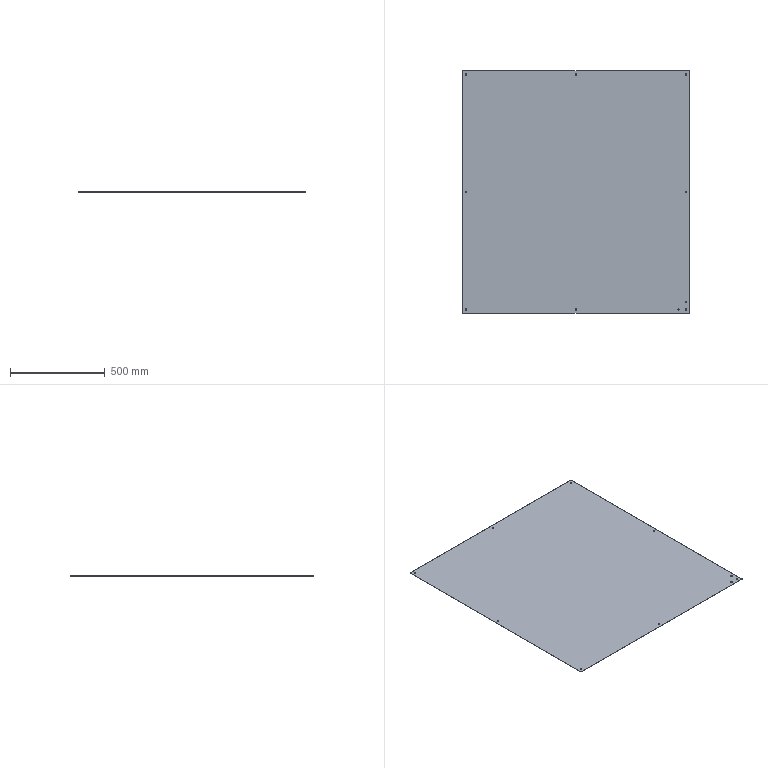Part | SolidWorks | features Fillet 2, HoleWzd 2, FlatPattern 1, SMBaseFlange 1, SheetMetal 1 | 1 solid | 30 faces | box 1200 x 1280 x 1.2 mm | volume 1842780 mm3 | cylinder 24 | plane 6 | commonest cylinder face diameters 6.6 x20 6 x4
STEP:
#1=CARTESIAN_POINT('',(576.7,-580.,-1.2));
#2=VERTEX_POINT('',#1);
#3=CARTESIAN_POINT('',(583.3,-580.,-1.2));
#4=VERTEX_POINT('',#3);
#5=CARTESIAN_POINT('',(580.,-580.,-1.2));
#6=DIRECTION('',(0.,0.,1.));
#7=DIRECTION('',(1.,0.,0.));
#8=AXIS2_PLACEMENT_3D('',#5,#6,#7);
#9=CIRCLE('',#8,3.3);
#10=EDGE_CURVE('',#2,#4,#9,.T.);
#11=ORIENTED_EDGE('',*,*,#10,.F.);
#12=CARTESIAN_POINT('',(576.7,-580.,0.));
#13=VERTEX_POINT('',#12);
#14=CARTESIAN_POINT('',(576.7,-580.,0.));
#15=DIRECTION('',(0.,0.,1.));
#16=VECTOR('',#15,1000.);
#17=LINE('',#14,#16);
#18=EDGE_CURVE('',#2,#13,#17,.T.);
#19=ORIENTED_EDGE('',*,*,#18,.T.);
#20=CARTESIAN_POINT('',(583.3,-580.,0.));
#21=VERTEX_POINT('',#20);
#22=CARTESIAN_POINT('',(580.,-580.,0.));
#23=DIRECTION('',(0.,0.,1.));
#24=DIRECTION('',(1.,0.,0.));
#25=AXIS2_PLACEMENT_3D('',#22,#23,#24);
#26=CIRCLE('',#25,3.3);
#27=EDGE_CURVE('',#13,#21,#26,.T.);
#28=ORIENTED_EDGE('',*,*,#27,.T.);
#29=CARTESIAN_POINT('',(583.3,-580.,0.));
#30=DIRECTION('',(0.,0.,1.));
#31=VECTOR('',#30,1000.);
#32=LINE('',#29,#31);
#33=EDGE_CURVE('',#4,#21,#32,.T.);
#34=ORIENTED_EDGE('',*,*,#33,.F.);
#35=EDGE_LOOP('',(#11,#19,#28,#34));
#36=FACE_OUTER_BOUND('',#35,.T.);
#37=CARTESIAN_POINT('',(580.,-580.,0.));
#38=DIRECTION('',(0.,0.,1.));
#39=DIRECTION('',(1.,0.,0.));
#40=AXIS2_PLACEMENT_3D('',#37,#38,#39);
#41=CYLINDRICAL_SURFACE('',#40,3.3);
#42=ADVANCED_FACE('',(#36),#41,.F.);
#43=CARTESIAN_POINT('',(536.7,-620.,-1.2));
#44=VERTEX_POINT('',#43);
#45=CARTESIAN_POINT('',(543.3,-620.,-1.2));
#46=VERTEX_POINT('',#45);
#47=CARTESIAN_POINT('',(540.,-620.,-1.2));
#48=DIRECTION('',(0.,0.,1.));
#49=DIRECTION('',(1.,0.,0.));
#50=AXIS2_PLACEMENT_3D('',#47,#48,#49);
#51=CIRCLE('',#50,3.3);
#52=EDGE_CURVE('',#44,#46,#51,.T.);
#53=ORIENTED_EDGE('',*,*,#52,.F.);
#54=CARTESIAN_POINT('',(536.7,-620.,0.));
#55=VERTEX_POINT('',#54);
#56=CARTESIAN_POINT('',(536.7,-620.,0.));
#57=DIRECTION('',(0.,0.,1.));
#58=VECTOR('',#57,1000.);
#59=LINE('',#56,#58);
#60=EDGE_CURVE('',#44,#55,#59,.T.);
#61=ORIENTED_EDGE('',*,*,#60,.T.);
#62=CARTESIAN_POINT('',(543.3,-620.,0.));
#63=VERTEX_POINT('',#62);
#64=CARTESIAN_POINT('',(540.,-620.,0.));
#65=DIRECTION('',(0.,0.,1.));
#66=DIRECTION('',(1.,0.,0.));
#67=AXIS2_PLACEMENT_3D('',#64,#65,#66);
#68=CIRCLE('',#67,3.3);
#69=EDGE_CURVE('',#55,#63,#68,.T.);
#70=ORIENTED_EDGE('',*,*,#69,.T.);
#71=CARTESIAN_POINT('',(543.3,-620.,0.));
#72=DIRECTION('',(0.,0.,1.));
#73=VECTOR('',#72,1000.);
#74=LINE('',#71,#73);
#75=EDGE_CURVE('',#46,#63,#74,.T.);
#76=ORIENTED_EDGE('',*,*,#75,.F.);
#77=EDGE_LOOP('',(#53,#61,#70,#76));
#78=FACE_OUTER_BOUND('',#77,.T.);
#79=CARTESIAN_POINT('',(540.,-620.,0.));
#80=DIRECTION('',(0.,0.,1.));
#81=DIRECTION('',(1.,0.,0.));
#82=AXIS2_PLACEMENT_3D('',#79,#80,#81);
#83=CYLINDRICAL_SURFACE('',#82,3.3);
#84=ADVANCED_FACE('',(#78),#83,.F.);
#85=CARTESIAN_POINT('',(-583.3,620.,-1.2));
#86=VERTEX_POINT('',#85);
#87=CARTESIAN_POINT('',(-576.7,620.,-1.2));
#88=VERTEX_POINT('',#87);
#89=CARTESIAN_POINT('',(-580.,620.,-1.2));
#90=DIRECTION('',(0.,0.,1.));
#91=DIRECTION('',(1.,0.,0.));
#92=AXIS2_PLACEMENT_3D('',#89,#90,#91);
#93=CIRCLE('',#92,3.3);
#94=EDGE_CURVE('',#86,#88,#93,.T.);
#95=ORIENTED_EDGE('',*,*,#94,.F.);
#96=CARTESIAN_POINT('',(-583.3,620.,0.));
#97=VERTEX_POINT('',#96);
#98=CARTESIAN_POINT('',(-583.3,620.,0.));
#99=DIRECTION('',(0.,0.,1.));
#100=VECTOR('',#99,1000.);
#101=LINE('',#98,#100);
#102=EDGE_CURVE('',#86,#97,#101,.T.);
#103=ORIENTED_EDGE('',*,*,#102,.T.);
#104=CARTESIAN_POINT('',(-576.7,620.,0.));
#105=VERTEX_POINT('',#104);
#106=CARTESIAN_POINT('',(-580.,620.,0.));
#107=DIRECTION('',(0.,0.,1.));
#108=DIRECTION('',(1.,0.,0.));
#109=AXIS2_PLACEMENT_3D('',#106,#107,#108);
#110=CIRCLE('',#109,3.3);
#111=EDGE_CURVE('',#97,#105,#110,.T.);
#112=ORIENTED_EDGE('',*,*,#111,.T.);
#113=CARTESIAN_POINT('',(-576.7,620.,0.));
#114=DIRECTION('',(0.,0.,1.));
#115=VECTOR('',#114,1000.);
#116=LINE('',#113,#115);
#117=EDGE_CURVE('',#88,#105,#116,.T.);
#118=ORIENTED_EDGE('',*,*,#117,.F.);
#119=EDGE_LOOP('',(#95,#103,#112,#118));
#120=FACE_OUTER_BOUND('',#119,.T.);
#121=CARTESIAN_POINT('',(-580.,620.,0.));
#122=DIRECTION('',(0.,0.,1.));
#123=DIRECTION('',(1.,0.,0.));
#124=AXIS2_PLACEMENT_3D('',#121,#122,#123);
#125=CYLINDRICAL_SURFACE('',#124,3.3);
#126=ADVANCED_FACE('',(#120),#125,.F.);
#127=CARTESIAN_POINT('',(-3.3,620.,-1.2));
#128=VERTEX_POINT('',#127);
#129=CARTESIAN_POINT('',(3.3,620.,-1.2));
#130=VERTEX_POINT('',#129);
#131=CARTESIAN_POINT('',(0.,620.,-1.2));
#132=DIRECTION('',(0.,0.,1.));
#133=DIRECTION('',(1.,0.,0.));
#134=AXIS2_PLACEMENT_3D('',#131,#132,#133);
#135=CIRCLE('',#134,3.3);
#136=EDGE_CURVE('',#128,#130,#135,.T.);
#137=ORIENTED_EDGE('',*,*,#136,.F.);
#138=CARTESIAN_POINT('',(-3.3,620.,0.));
#139=VERTEX_POINT('',#138);
#140=CARTESIAN_POINT('',(-3.3,620.,0.));
#141=DIRECTION('',(0.,0.,1.));
#142=VECTOR('',#141,1000.);
#143=LINE('',#140,#142);
#144=EDGE_CURVE('',#128,#139,#143,.T.);
#145=ORIENTED_EDGE('',*,*,#144,.T.);
#146=CARTESIAN_POINT('',(3.3,620.,0.));
#147=VERTEX_POINT('',#146);
#148=CARTESIAN_POINT('',(0.,620.,0.));
#149=DIRECTION('',(0.,0.,1.));
#150=DIRECTION('',(1.,0.,0.));
#151=AXIS2_PLACEMENT_3D('',#148,#149,#150);
#152=CIRCLE('',#151,3.3);
#153=EDGE_CURVE('',#139,#147,#152,.T.);
#154=ORIENTED_EDGE('',*,*,#153,.T.);
#155=CARTESIAN_POINT('',(3.3,620.,0.));
#156=DIRECTION('',(0.,0.,1.));
#157=VECTOR('',#156,1000.);
#158=LINE('',#155,#157);
#159=EDGE_CURVE('',#130,#147,#158,.T.);
#160=ORIENTED_EDGE('',*,*,#159,.F.);
#161=EDGE_LOOP('',(#137,#145,#154,#160));
#162=FACE_OUTER_BOUND('',#161,.T.);
#163=CARTESIAN_POINT('',(0.,620.,0.));
#164=DIRECTION('',(0.,0.,1.));
#165=DIRECTION('',(1.,0.,0.));
#166=AXIS2_PLACEMENT_3D('',#163,#164,#165);
#167=CYLINDRICAL_SURFACE('',#166,3.3);
#168=ADVANCED_FACE('',(#162),#167,.F.);
#169=CARTESIAN_POINT('',(576.7,620.,-1.2));
#170=VERTEX_POINT('',#169);
#171=CARTESIAN_POINT('',(583.3,620.,-1.2));
#172=VERTEX_POINT('',#171);
#173=CARTESIAN_POINT('',(580.,620.,-1.2));
#174=DIRECTION('',(0.,0.,1.));
#175=DIRECTION('',(1.,0.,0.));
#176=AXIS2_PLACEMENT_3D('',#173,#174,#175);
#177=CIRCLE('',#176,3.3);
#178=EDGE_CURVE('',#170,#172,#177,.T.);
#179=ORIENTED_EDGE('',*,*,#178,.F.);
#180=CARTESIAN_POINT('',(576.7,620.,0.));
#181=VERTEX_POINT('',#180);
#182=CARTESIAN_POINT('',(576.7,620.,0.));
#183=DIRECTION('',(0.,0.,1.));
#184=VECTOR('',#183,1000.);
#185=LINE('',#182,#184);
#186=EDGE_CURVE('',#170,#181,#185,.T.);
#187=ORIENTED_EDGE('',*,*,#186,.T.);
#188=CARTESIAN_POINT('',(583.3,620.,0.));
#189=VERTEX_POINT('',#188);
#190=CARTESIAN_POINT('',(580.,620.,0.));
#191=DIRECTION('',(0.,0.,1.));
#192=DIRECTION('',(1.,0.,0.));
#193=AXIS2_PLACEMENT_3D('',#190,#191,#192);
#194=CIRCLE('',#193,3.3);
#195=EDGE_CURVE('',#181,#189,#194,.T.);
#196=ORIENTED_EDGE('',*,*,#195,.T.);
#197=CARTESIAN_POINT('',(583.3,620.,0.));
#198=DIRECTION('',(0.,0.,1.));
#199=VECTOR('',#198,1000.);
#200=LINE('',#197,#199);
#201=EDGE_CURVE('',#172,#189,#200,.T.);
#202=ORIENTED_EDGE('',*,*,#201,.F.);
#203=EDGE_LOOP('',(#179,#187,#196,#202));
#204=FACE_OUTER_BOUND('',#203,.T.);
#205=CARTESIAN_POINT('',(580.,620.,0.));
#206=DIRECTION('',(0.,0.,1.));
#207=DIRECTION('',(1.,0.,0.));
#208=AXIS2_PLACEMENT_3D('',#205,#206,#207);
#209=CYLINDRICAL_SURFACE('',#208,3.3);
#210=ADVANCED_FACE('',(#204),#209,.F.);
#211=CARTESIAN_POINT('',(576.7,0.,-1.2));
#212=VERTEX_POINT('',#211);
#213=CARTESIAN_POINT('',(583.3,0.,-1.2));
#214=VERTEX_POINT('',#213);
#215=CARTESIAN_POINT('',(580.,0.,-1.2));
#216=DIRECTION('',(0.,0.,1.));
#217=DIRECTION('',(1.,0.,0.));
#218=AXIS2_PLACEMENT_3D('',#215,#216,#217);
#219=CIRCLE('',#218,3.3);
#220=EDGE_CURVE('',#212,#214,#219,.T.);
#221=ORIENTED_EDGE('',*,*,#220,.F.);
#222=CARTESIAN_POINT('',(576.7,0.,0.));
#223=VERTEX_POINT('',#222);
#224=CARTESIAN_POINT('',(576.7,0.,0.));
#225=DIRECTION('',(0.,0.,1.));
#226=VECTOR('',#225,1000.);
#227=LINE('',#224,#226);
#228=EDGE_CURVE('',#212,#223,#227,.T.);
#229=ORIENTED_EDGE('',*,*,#228,.T.);
#230=CARTESIAN_POINT('',(583.3,0.,0.));
#231=VERTEX_POINT('',#230);
#232=CARTESIAN_POINT('',(580.,0.,0.));
#233=DIRECTION('',(0.,0.,1.));
#234=DIRECTION('',(1.,0.,0.));
#235=AXIS2_PLACEMENT_3D('',#232,#233,#234);
#236=CIRCLE('',#235,3.3);
#237=EDGE_CURVE('',#223,#231,#236,.T.);
#238=ORIENTED_EDGE('',*,*,#237,.T.);
#239=CARTESIAN_POINT('',(583.3,0.,0.));
#240=DIRECTION('',(0.,0.,1.));
#241=VECTOR('',#240,1000.);
#242=LINE('',#239,#241);
#243=EDGE_CURVE('',#214,#231,#242,.T.);
#244=ORIENTED_EDGE('',*,*,#243,.F.);
#245=EDGE_LOOP('',(#221,#229,#238,#244));
#246=FACE_OUTER_BOUND('',#245,.T.);
#247=CARTESIAN_POINT('',(580.,0.,0.));
#248=DIRECTION('',(0.,0.,1.));
#249=DIRECTION('',(1.,0.,0.));
#250=AXIS2_PLACEMENT_3D('',#247,#248,#249);
#251=CYLINDRICAL_SURFACE('',#250,3.3);
#252=ADVANCED_FACE('',(#246),#251,.F.);
#253=CARTESIAN_POINT('',(576.7,-620.,-1.2));
#254=VERTEX_POINT('',#253);
#255=CARTESIAN_POINT('',(583.3,-620.,-1.2));
#256=VERTEX_POINT('',#255);
#257=CARTESIAN_POINT('',(580.,-620.,-1.2));
#258=DIRECTION('',(0.,0.,1.));
#259=DIRECTION('',(1.,0.,0.));
#260=AXIS2_PLACEMENT_3D('',#257,#258,#259);
#261=CIRCLE('',#260,3.3);
#262=EDGE_CURVE('',#254,#256,#261,.T.);
#263=ORIENTED_EDGE('',*,*,#262,.F.);
#264=CARTESIAN_POINT('',(576.7,-620.,0.));
#265=VERTEX_POINT('',#264);
#266=CARTESIAN_POINT('',(576.7,-620.,0.));
#267=DIRECTION('',(0.,0.,1.));
#268=VECTOR('',#267,1000.);
#269=LINE('',#266,#268);
#270=EDGE_CURVE('',#254,#265,#269,.T.);
#271=ORIENTED_EDGE('',*,*,#270,.T.);
#272=CARTESIAN_POINT('',(583.3,-620.,0.));
#273=VERTEX_POINT('',#272);
#274=CARTESIAN_POINT('',(580.,-620.,0.));
#275=DIRECTION('',(0.,0.,1.));
#276=DIRECTION('',(1.,0.,0.));
#277=AXIS2_PLACEMENT_3D('',#274,#275,#276);
#278=CIRCLE('',#277,3.3);
#279=EDGE_CURVE('',#265,#273,#278,.T.);
#280=ORIENTED_EDGE('',*,*,#279,.T.);
#281=CARTESIAN_POINT('',(583.3,-620.,0.));
#282=DIRECTION('',(0.,0.,1.));
#283=VECTOR('',#282,1000.);
#284=LINE('',#281,#283);
#285=EDGE_CURVE('',#256,#273,#284,.T.);
#286=ORIENTED_EDGE('',*,*,#285,.F.);
#287=EDGE_LOOP('',(#263,#271,#280,#286));
#288=FACE_OUTER_BOUND('',#287,.T.);
#289=CARTESIAN_POINT('',(580.,-620.,0.));
#290=DIRECTION('',(0.,0.,1.));
#291=DIRECTION('',(1.,0.,0.));
#292=AXIS2_PLACEMENT_3D('',#289,#290,#291);
#293=CYLINDRICAL_SURFACE('',#292,3.3);
#294=ADVANCED_FACE('',(#288),#293,.F.);
#295=CARTESIAN_POINT('',(-3.3,-620.,-1.2));
#296=VERTEX_POINT('',#295);
#297=CARTESIAN_POINT('',(3.3,-620.,-1.2));
#298=VERTEX_POINT('',#297);
#299=CARTESIAN_POINT('',(0.,-620.,-1.2));
#300=DIRECTION('',(0.,0.,1.));
#301=DIRECTION('',(1.,0.,0.));
#302=AXIS2_PLACEMENT_3D('',#299,#300,#301);
#303=CIRCLE('',#302,3.3);
#304=EDGE_CURVE('',#296,#298,#303,.T.);
#305=ORIENTED_EDGE('',*,*,#304,.F.);
#306=CARTESIAN_POINT('',(-3.3,-620.,0.));
#307=VERTEX_POINT('',#306);
#308=CARTESIAN_POINT('',(-3.3,-620.,0.));
#309=DIRECTION('',(0.,0.,1.));
#310=VECTOR('',#309,1000.);
#311=LINE('',#308,#310);
#312=EDGE_CURVE('',#296,#307,#311,.T.);
#313=ORIENTED_EDGE('',*,*,#312,.T.);
#314=CARTESIAN_POINT('',(3.3,-620.,0.));
#315=VERTEX_POINT('',#314);
#316=CARTESIAN_POINT('',(0.,-620.,0.));
#317=DIRECTION('',(0.,0.,1.));
#318=DIRECTION('',(1.,0.,0.));
#319=AXIS2_PLACEMENT_3D('',#316,#317,#318);
#320=CIRCLE('',#319,3.3);
#321=EDGE_CURVE('',#307,#315,#320,.T.);
#322=ORIENTED_EDGE('',*,*,#321,.T.);
#323=CARTESIAN_POINT('',(3.3,-620.,0.));
#324=DIRECTION('',(0.,0.,1.));
#325=VECTOR('',#324,1000.);
#326=LINE('',#323,#325);
#327=EDGE_CURVE('',#298,#315,#326,.T.);
#328=ORIENTED_EDGE('',*,*,#327,.F.);
#329=EDGE_LOOP('',(#305,#313,#322,#328));
#330=FACE_OUTER_BOUND('',#329,.T.);
#331=CARTESIAN_POINT('',(0.,-620.,0.));
#332=DIRECTION('',(0.,0.,1.));
#333=DIRECTION('',(1.,0.,0.));
#334=AXIS2_PLACEMENT_3D('',#331,#332,#333);
#335=CYLINDRICAL_SURFACE('',#334,3.3);
#336=ADVANCED_FACE('',(#330),#335,.F.);
#337=CARTESIAN_POINT('',(-583.3,-620.,-1.2));
#338=VERTEX_POINT('',#337);
#339=CARTESIAN_POINT('',(-576.7,-620.,-1.2));
#340=VERTEX_POINT('',#339);
#341=CARTESIAN_POINT('',(-580.,-620.,-1.2));
#342=DIRECTION('',(0.,0.,1.));
#343=DIRECTION('',(1.,0.,0.));
#344=AXIS2_PLACEMENT_3D('',#341,#342,#343);
#345=CIRCLE('',#344,3.3);
#346=EDGE_CURVE('',#338,#340,#345,.T.);
#347=ORIENTED_EDGE('',*,*,#346,.F.);
#348=CARTESIAN_POINT('',(-583.3,-620.,0.));
#349=VERTEX_POINT('',#348);
#350=CARTESIAN_POINT('',(-583.3,-620.,0.));
#351=DIRECTION('',(0.,0.,1.));
#352=VECTOR('',#351,1000.);
#353=LINE('',#350,#352);
#354=EDGE_CURVE('',#338,#349,#353,.T.);
#355=ORIENTED_EDGE('',*,*,#354,.T.);
#356=CARTESIAN_POINT('',(-576.7,-620.,0.));
#357=VERTEX_POINT('',#356);
#358=CARTESIAN_POINT('',(-580.,-620.,0.));
#359=DIRECTION('',(0.,0.,1.));
#360=DIRECTION('',(1.,0.,0.));
#361=AXIS2_PLACEMENT_3D('',#358,#359,#360);
#362=CIRCLE('',#361,3.3);
#363=EDGE_CURVE('',#349,#357,#362,.T.);
#364=ORIENTED_EDGE('',*,*,#363,.T.);
#365=CARTESIAN_POINT('',(-576.7,-620.,0.));
#366=DIRECTION('',(0.,0.,1.));
#367=VECTOR('',#366,1000.);
#368=LINE('',#365,#367);
#369=EDGE_CURVE('',#340,#357,#368,.T.);
#370=ORIENTED_EDGE('',*,*,#369,.F.);
#371=EDGE_LOOP('',(#347,#355,#364,#370));
#372=FACE_OUTER_BOUND('',#371,.T.);
#373=CARTESIAN_POINT('',(-580.,-620.,0.));
#374=DIRECTION('',(0.,0.,1.));
#375=DIRECTION('',(1.,0.,0.));
#376=AXIS2_PLACEMENT_3D('',#373,#374,#375);
#377=CYLINDRICAL_SURFACE('',#376,3.3);
#378=ADVANCED_FACE('',(#372),#377,.F.);
#379=CARTESIAN_POINT('',(-583.3,0.,-1.2));
#380=VERTEX_POINT('',#379);
#381=CARTESIAN_POINT('',(-576.7,0.,-1.2));
#382=VERTEX_POINT('',#381);
#383=CARTESIAN_POINT('',(-580.,0.,-1.2));
#384=DIRECTION('',(0.,0.,1.));
#385=DIRECTION('',(1.,0.,0.));
#386=AXIS2_PLACEMENT_3D('',#383,#384,#385);
#387=CIRCLE('',#386,3.3);
#388=EDGE_CURVE('',#380,#382,#387,.T.);
#389=ORIENTED_EDGE('',*,*,#388,.F.);
#390=CARTESIAN_POINT('',(-583.3,0.,0.));
#391=VERTEX_POINT('',#390);
#392=CARTESIAN_POINT('',(-583.3,0.,0.));
#393=DIRECTION('',(0.,0.,1.));
#394=VECTOR('',#393,1000.);
#395=LINE('',#392,#394);
#396=EDGE_CURVE('',#380,#391,#395,.T.);
#397=ORIENTED_EDGE('',*,*,#396,.T.);
#398=CARTESIAN_POINT('',(-576.7,0.,0.));
#399=VERTEX_POINT('',#398);
#400=CARTESIAN_POINT('',(-580.,0.,0.));
#401=DIRECTION('',(0.,0.,1.));
#402=DIRECTION('',(1.,0.,0.));
#403=AXIS2_PLACEMENT_3D('',#400,#401,#402);
#404=CIRCLE('',#403,3.3);
#405=EDGE_CURVE('',#391,#399,#404,.T.);
#406=ORIENTED_EDGE('',*,*,#405,.T.);
#407=CARTESIAN_POINT('',(-576.7,0.,0.));
#408=DIRECTION('',(0.,0.,1.));
#409=VECTOR('',#408,1000.);
#410=LINE('',#407,#409);
#411=EDGE_CURVE('',#382,#399,#410,.T.);
#412=ORIENTED_EDGE('',*,*,#411,.F.);
#413=EDGE_LOOP('',(#389,#397,#406,#412));
#414=FACE_OUTER_BOUND('',#413,.T.);
#415=CARTESIAN_POINT('',(-580.,0.,0.));
#416=DIRECTION('',(0.,0.,1.));
#417=DIRECTION('',(1.,0.,0.));
#418=AXIS2_PLACEMENT_3D('',#415,#416,#417);
#419=CYLINDRICAL_SURFACE('',#418,3.3);
#420=ADVANCED_FACE('',(#414),#419,.F.);
#421=CARTESIAN_POINT('',(600.,-637.,-1.2));
#422=VERTEX_POINT('',#421);
#423=CARTESIAN_POINT('',(600.,637.,-1.2));
#424=VERTEX_POINT('',#423);
#425=CARTESIAN_POINT('',(600.,640.,-1.2));
#426=DIRECTION('',(0.,1.,0.));
#427=VECTOR('',#426,1000.);
#428=LINE('',#425,#427);
#429=EDGE_CURVE('',#422,#424,#428,.T.);
#430=ORIENTED_EDGE('',*,*,#429,.T.);
#431=CARTESIAN_POINT('',(600.,637.,0.));
#432=VERTEX_POINT('',#431);
#433=CARTESIAN_POINT('',(600.,637.,-1.2));
#434=DIRECTION('',(0.,0.,1.));
#435=VECTOR('',#434,1000.);
#436=LINE('',#433,#435);
#437=EDGE_CURVE('',#424,#432,#436,.T.);
#438=ORIENTED_EDGE('',*,*,#437,.T.);
#439=CARTESIAN_POINT('',(600.,-637.,0.));
#440=VERTEX_POINT('',#439);
#441=CARTESIAN_POINT('',(600.,640.,0.));
#442=DIRECTION('',(0.,1.,0.));
#443=VECTOR('',#442,1000.);
#444=LINE('',#441,#443);
#445=EDGE_CURVE('',#440,#432,#444,.T.);
#446=ORIENTED_EDGE('',*,*,#445,.F.);
#447=CARTESIAN_POINT('',(600.,-637.,-1.2));
#448=DIRECTION('',(0.,0.,-1.));
#449=VECTOR('',#448,1000.);
#450=LINE('',#447,#449);
#451=EDGE_CURVE('',#440,#422,#450,.T.);
#452=ORIENTED_EDGE('',*,*,#451,.T.);
#453=EDGE_LOOP('',(#430,#438,#446,#452));
#454=FACE_OUTER_BOUND('',#453,.T.);
#455=CARTESIAN_POINT('',(600.,640.,-1.2));
#456=DIRECTION('',(1.,0.,0.));
#457=DIRECTION('',(0.,0.,-1.));
#458=AXIS2_PLACEMENT_3D('',#455,#456,#457);
#459=PLANE('',#458);
#460=ADVANCED_FACE('',(#454),#459,.T.);
#461=CARTESIAN_POINT('',(-597.,-640.,-1.2));
#462=VERTEX_POINT('',#461);
#463=CARTESIAN_POINT('',(597.,-640.,-1.2));
#464=VERTEX_POINT('',#463);
#465=CARTESIAN_POINT('',(-600.,-640.,-1.2));
#466=DIRECTION('',(1.,0.,0.));
#467=VECTOR('',#466,1000.);
#468=LINE('',#465,#467);
#469=EDGE_CURVE('',#462,#464,#468,.T.);
#470=ORIENTED_EDGE('',*,*,#469,.T.);
#471=CARTESIAN_POINT('',(597.,-640.,0.));
#472=VERTEX_POINT('',#471);
#473=CARTESIAN_POINT('',(597.,-640.,-1.2));
#474=DIRECTION('',(0.,0.,1.));
#475=VECTOR('',#474,1000.);
#476=LINE('',#473,#475);
#477=EDGE_CURVE('',#464,#472,#476,.T.);
#478=ORIENTED_EDGE('',*,*,#477,.T.);
#479=CARTESIAN_POINT('',(-597.,-640.,0.));
#480=VERTEX_POINT('',#479);
#481=CARTESIAN_POINT('',(-600.,-640.,0.));
#482=DIRECTION('',(1.,0.,0.));
#483=VECTOR('',#482,1000.);
#484=LINE('',#481,#483);
#485=EDGE_CURVE('',#480,#472,#484,.T.);
#486=ORIENTED_EDGE('',*,*,#485,.F.);
#487=CARTESIAN_POINT('',(-597.,-640.,-1.2));
#488=DIRECTION('',(0.,0.,-1.));
#489=VECTOR('',#488,1000.);
#490=LINE('',#487,#489);
#491=EDGE_CURVE('',#480,#462,#490,.T.);
#492=ORIENTED_EDGE('',*,*,#491,.T.);
#493=EDGE_LOOP('',(#470,#478,#486,#492));
#494=FACE_OUTER_BOUND('',#493,.T.);
#495=CARTESIAN_POINT('',(-600.,-640.,-1.2));
#496=DIRECTION('',(0.,-1.,0.));
#497=DIRECTION('',(0.,0.,-1.));
#498=AXIS2_PLACEMENT_3D('',#495,#496,#497);
#499=PLANE('',#498);
#500=ADVANCED_FACE('',(#494),#499,.T.);
#501=CARTESIAN_POINT('',(-600.,637.,0.));
#502=VERTEX_POINT('',#501);
#503=CARTESIAN_POINT('',(-600.,-637.,0.));
#504=VERTEX_POINT('',#503);
#505=CARTESIAN_POINT('',(-600.,640.,0.));
#506=DIRECTION('',(0.,-1.,0.));
#507=VECTOR('',#506,1000.);
#508=LINE('',#505,#507);
#509=EDGE_CURVE('',#502,#504,#508,.T.);
#510=ORIENTED_EDGE('',*,*,#509,.F.);
#511=CARTESIAN_POINT('',(-600.,637.,-1.2));
#512=VERTEX_POINT('',#511);
#513=CARTESIAN_POINT('',(-600.,637.,-1.2));
#514=DIRECTION('',(0.,0.,-1.));
#515=VECTOR('',#514,1000.);
#516=LINE('',#513,#515);
#517=EDGE_CURVE('',#502,#512,#516,.T.);
#518=ORIENTED_EDGE('',*,*,#517,.T.);
#519=CARTESIAN_POINT('',(-600.,-637.,-1.2));
#520=VERTEX_POINT('',#519);
#521=CARTESIAN_POINT('',(-600.,640.,-1.2));
#522=DIRECTION('',(0.,-1.,0.));
#523=VECTOR('',#522,1000.);
#524=LINE('',#521,#523);
#525=EDGE_CURVE('',#512,#520,#524,.T.);
#526=ORIENTED_EDGE('',*,*,#525,.T.);
#527=CARTESIAN_POINT('',(-600.,-637.,-1.2));
#528=DIRECTION('',(0.,0.,1.));
#529=VECTOR('',#528,1000.);
#530=LINE('',#527,#529);
#531=EDGE_CURVE('',#520,#504,#530,.T.);
#532=ORIENTED_EDGE('',*,*,#531,.T.);
#533=EDGE_LOOP('',(#510,#518,#526,#532));
#534=FACE_OUTER_BOUND('',#533,.T.);
#535=CARTESIAN_POINT('',(-600.,640.,-1.2));
#536=DIRECTION('',(-1.,0.,0.));
#537=DIRECTION('',(0.,-1.,0.));
#538=AXIS2_PLACEMENT_3D('',#535,#536,#537);
#539=PLANE('',#538);
#540=ADVANCED_FACE('',(#534),#539,.T.);
#541=CARTESIAN_POINT('',(597.,640.,-1.2));
#542=VERTEX_POINT('',#541);
#543=CARTESIAN_POINT('',(-597.,640.,-1.2));
#544=VERTEX_POINT('',#543);
#545=CARTESIAN_POINT('',(-600.,640.,-1.2));
#546=DIRECTION('',(-1.,0.,0.));
#547=VECTOR('',#546,1000.);
#548=LINE('',#545,#547);
#549=EDGE_CURVE('',#542,#544,#548,.T.);
#550=ORIENTED_EDGE('',*,*,#549,.T.);
#551=CARTESIAN_POINT('',(-597.,640.,0.));
#552=VERTEX_POINT('',#551);
#553=CARTESIAN_POINT('',(-597.,640.,-1.2));
#554=DIRECTION('',(0.,0.,1.));
#555=VECTOR('',#554,1000.);
#556=LINE('',#553,#555);
#557=EDGE_CURVE('',#544,#552,#556,.T.);
#558=ORIENTED_EDGE('',*,*,#557,.T.);
#559=CARTESIAN_POINT('',(597.,640.,0.));
#560=VERTEX_POINT('',#559);
#561=CARTESIAN_POINT('',(-600.,640.,0.));
#562=DIRECTION('',(-1.,0.,0.));
#563=VECTOR('',#562,1000.);
#564=LINE('',#561,#563);
#565=EDGE_CURVE('',#560,#552,#564,.T.);
#566=ORIENTED_EDGE('',*,*,#565,.F.);
#567=CARTESIAN_POINT('',(597.,640.,-1.2));
#568=DIRECTION('',(0.,0.,-1.));
#569=VECTOR('',#568,1000.);
#570=LINE('',#567,#569);
#571=EDGE_CURVE('',#560,#542,#570,.T.);
#572=ORIENTED_EDGE('',*,*,#571,.T.);
#573=EDGE_LOOP('',(#550,#558,#566,#572));
#574=FACE_OUTER_BOUND('',#573,.T.);
#575=CARTESIAN_POINT('',(-600.,640.,-1.2));
#576=DIRECTION('',(0.,1.,0.));
#577=DIRECTION('',(0.,0.,1.));
#578=AXIS2_PLACEMENT_3D('',#575,#576,#577);
#579=PLANE('',#578);
#580=ADVANCED_FACE('',(#574),#579,.T.);
#581=CARTESIAN_POINT('',(580.,-580.,-1.2));
#582=DIRECTION('',(0.,0.,1.));
#583=DIRECTION('',(1.,0.,0.));
#584=AXIS2_PLACEMENT_3D('',#581,#582,#583);
#585=CIRCLE('',#584,3.3);
#586=EDGE_CURVE('',#4,#2,#585,.T.);
#587=ORIENTED_EDGE('',*,*,#586,.T.);
#588=ORIENTED_EDGE('',*,*,#10,.T.);
#589=EDGE_LOOP('',(#587,#588));
#590=FACE_BOUND('',#589,.T.);
#591=CARTESIAN_POINT('',(540.,-620.,-1.2));
#592=DIRECTION('',(0.,0.,1.));
#593=DIRECTION('',(1.,0.,0.));
#594=AXIS2_PLACEMENT_3D('',#591,#592,#593);
#595=CIRCLE('',#594,3.3);
#596=EDGE_CURVE('',#46,#44,#595,.T.);
#597=ORIENTED_EDGE('',*,*,#596,.T.);
#598=ORIENTED_EDGE('',*,*,#52,.T.);
#599=EDGE_LOOP('',(#597,#598));
#600=FACE_BOUND('',#599,.T.);
#601=CARTESIAN_POINT('',(-580.,620.,-1.2));
#602=DIRECTION('',(0.,0.,1.));
#603=DIRECTION('',(1.,0.,0.));
#604=AXIS2_PLACEMENT_3D('',#601,#602,#603);
#605=CIRCLE('',#604,3.3);
#606=EDGE_CURVE('',#88,#86,#605,.T.);
#607=ORIENTED_EDGE('',*,*,#606,.T.);
#608=ORIENTED_EDGE('',*,*,#94,.T.);
#609=EDGE_LOOP('',(#607,#608));
#610=FACE_BOUND('',#609,.T.);
#611=CARTESIAN_POINT('',(0.,620.,-1.2));
#612=DIRECTION('',(0.,0.,1.));
#613=DIRECTION('',(1.,0.,0.));
#614=AXIS2_PLACEMENT_3D('',#611,#612,#613);
#615=CIRCLE('',#614,3.3);
#616=EDGE_CURVE('',#130,#128,#615,.T.);
#617=ORIENTED_EDGE('',*,*,#616,.T.);
#618=ORIENTED_EDGE('',*,*,#136,.T.);
#619=EDGE_LOOP('',(#617,#618));
#620=FACE_BOUND('',#619,.T.);
#621=CARTESIAN_POINT('',(580.,620.,-1.2));
#622=DIRECTION('',(0.,0.,1.));
#623=DIRECTION('',(1.,0.,0.));
#624=AXIS2_PLACEMENT_3D('',#621,#622,#623);
#625=CIRCLE('',#624,3.3);
#626=EDGE_CURVE('',#172,#170,#625,.T.);
#627=ORIENTED_EDGE('',*,*,#626,.T.);
#628=ORIENTED_EDGE('',*,*,#178,.T.);
#629=EDGE_LOOP('',(#627,#628));
#630=FACE_BOUND('',#629,.T.);
#631=CARTESIAN_POINT('',(580.,0.,-1.2));
#632=DIRECTION('',(0.,0.,1.));
#633=DIRECTION('',(1.,0.,0.));
#634=AXIS2_PLACEMENT_3D('',#631,#632,#633);
#635=CIRCLE('',#634,3.3);
#636=EDGE_CURVE('',#214,#212,#635,.T.);
#637=ORIENTED_EDGE('',*,*,#636,.T.);
#638=ORIENTED_EDGE('',*,*,#220,.T.);
#639=EDGE_LOOP('',(#637,#638));
#640=FACE_BOUND('',#639,.T.);
#641=CARTESIAN_POINT('',(580.,-620.,-1.2));
#642=DIRECTION('',(0.,0.,1.));
#643=DIRECTION('',(1.,0.,0.));
#644=AXIS2_PLACEMENT_3D('',#641,#642,#643);
#645=CIRCLE('',#644,3.3);
#646=EDGE_CURVE('',#256,#254,#645,.T.);
#647=ORIENTED_EDGE('',*,*,#646,.T.);
#648=ORIENTED_EDGE('',*,*,#262,.T.);
#649=EDGE_LOOP('',(#647,#648));
#650=FACE_BOUND('',#649,.T.);
#651=CARTESIAN_POINT('',(0.,-620.,-1.2));
#652=DIRECTION('',(0.,0.,1.));
#653=DIRECTION('',(1.,0.,0.));
#654=AXIS2_PLACEMENT_3D('',#651,#652,#653);
#655=CIRCLE('',#654,3.3);
#656=EDGE_CURVE('',#298,#296,#655,.T.);
#657=ORIENTED_EDGE('',*,*,#656,.T.);
#658=ORIENTED_EDGE('',*,*,#304,.T.);
#659=EDGE_LOOP('',(#657,#658));
#660=FACE_BOUND('',#659,.T.);
#661=CARTESIAN_POINT('',(-580.,-620.,-1.2));
#662=DIRECTION('',(0.,0.,1.));
#663=DIRECTION('',(1.,0.,0.));
#664=AXIS2_PLACEMENT_3D('',#661,#662,#663);
#665=CIRCLE('',#664,3.3);
#666=EDGE_CURVE('',#340,#338,#665,.T.);
#667=ORIENTED_EDGE('',*,*,#666,.T.);
#668=ORIENTED_EDGE('',*,*,#346,.T.);
#669=EDGE_LOOP('',(#667,#668));
#670=FACE_BOUND('',#669,.T.);
#671=CARTESIAN_POINT('',(-580.,0.,-1.2));
#672=DIRECTION('',(0.,0.,1.));
#673=DIRECTION('',(1.,0.,0.));
#674=AXIS2_PLACEMENT_3D('',#671,#672,#673);
#675=CIRCLE('',#674,3.3);
#676=EDGE_CURVE('',#382,#380,#675,.T.);
#677=ORIENTED_EDGE('',*,*,#676,.T.);
#678=ORIENTED_EDGE('',*,*,#388,.T.);
#679=EDGE_LOOP('',(#677,#678));
#680=FACE_BOUND('',#679,.T.);
#681=ORIENTED_EDGE('',*,*,#525,.F.);
#682=CARTESIAN_POINT('',(-597.,637.,-1.2));
#683=DIRECTION('',(0.,0.,-1.));
#684=DIRECTION('',(1.,0.,0.));
#685=AXIS2_PLACEMENT_3D('',#682,#683,#684);
#686=CIRCLE('',#685,3.);
#687=EDGE_CURVE('',#512,#544,#686,.T.);
#688=ORIENTED_EDGE('',*,*,#687,.T.);
#689=ORIENTED_EDGE('',*,*,#549,.F.);
#690=CARTESIAN_POINT('',(597.,637.,-1.2));
#691=DIRECTION('',(0.,0.,-1.));
#692=DIRECTION('',(1.,0.,0.));
#693=AXIS2_PLACEMENT_3D('',#690,#691,#692);
#694=CIRCLE('',#693,3.);
#695=EDGE_CURVE('',#542,#424,#694,.T.);
#696=ORIENTED_EDGE('',*,*,#695,.T.);
#697=ORIENTED_EDGE('',*,*,#429,.F.);
#698=CARTESIAN_POINT('',(597.,-637.,-1.2));
#699=DIRECTION('',(0.,0.,-1.));
#700=DIRECTION('',(1.,0.,0.));
#701=AXIS2_PLACEMENT_3D('',#698,#699,#700);
#702=CIRCLE('',#701,3.);
#703=EDGE_CURVE('',#422,#464,#702,.T.);
#704=ORIENTED_EDGE('',*,*,#703,.T.);
#705=ORIENTED_EDGE('',*,*,#469,.F.);
#706=CARTESIAN_POINT('',(-597.,-637.,-1.2));
#707=DIRECTION('',(0.,0.,-1.));
#708=DIRECTION('',(1.,0.,0.));
#709=AXIS2_PLACEMENT_3D('',#706,#707,#708);
#710=CIRCLE('',#709,3.);
#711=EDGE_CURVE('',#462,#520,#710,.T.);
#712=ORIENTED_EDGE('',*,*,#711,.T.);
#713=EDGE_LOOP('',(#681,#688,#689,#696,#697,#704,#705,#712));
#714=FACE_OUTER_BOUND('',#713,.T.);
#715=CARTESIAN_POINT('',(0.,0.,-1.2));
#716=DIRECTION('',(0.,0.,1.));
#717=DIRECTION('',(1.,0.,0.));
#718=AXIS2_PLACEMENT_3D('',#715,#716,#717);
#719=PLANE('',#718);
#720=ADVANCED_FACE('',(#590,#600,#610,#620,#630,#640,#650,#660,#670,#680,#714),#719,.F.);
#721=CARTESIAN_POINT('',(580.,-580.,0.));
#722=DIRECTION('',(0.,0.,1.));
#723=DIRECTION('',(1.,0.,0.));
#724=AXIS2_PLACEMENT_3D('',#721,#722,#723);
#725=CIRCLE('',#724,3.3);
#726=EDGE_CURVE('',#21,#13,#725,.T.);
#727=ORIENTED_EDGE('',*,*,#726,.F.);
#728=ORIENTED_EDGE('',*,*,#27,.F.);
#729=EDGE_LOOP('',(#727,#728));
#730=FACE_BOUND('',#729,.T.);
#731=CARTESIAN_POINT('',(540.,-620.,0.));
#732=DIRECTION('',(0.,0.,1.));
#733=DIRECTION('',(1.,0.,0.));
#734=AXIS2_PLACEMENT_3D('',#731,#732,#733);
#735=CIRCLE('',#734,3.3);
#736=EDGE_CURVE('',#63,#55,#735,.T.);
#737=ORIENTED_EDGE('',*,*,#736,.F.);
#738=ORIENTED_EDGE('',*,*,#69,.F.);
#739=EDGE_LOOP('',(#737,#738));
#740=FACE_BOUND('',#739,.T.);
#741=CARTESIAN_POINT('',(-580.,620.,0.));
#742=DIRECTION('',(0.,0.,1.));
#743=DIRECTION('',(1.,0.,0.));
#744=AXIS2_PLACEMENT_3D('',#741,#742,#743);
#745=CIRCLE('',#744,3.3);
#746=EDGE_CURVE('',#105,#97,#745,.T.);
#747=ORIENTED_EDGE('',*,*,#746,.F.);
#748=ORIENTED_EDGE('',*,*,#111,.F.);
#749=EDGE_LOOP('',(#747,#748));
#750=FACE_BOUND('',#749,.T.);
#751=CARTESIAN_POINT('',(0.,620.,0.));
#752=DIRECTION('',(0.,0.,1.));
#753=DIRECTION('',(1.,0.,0.));
#754=AXIS2_PLACEMENT_3D('',#751,#752,#753);
#755=CIRCLE('',#754,3.3);
#756=EDGE_CURVE('',#147,#139,#755,.T.);
#757=ORIENTED_EDGE('',*,*,#756,.F.);
#758=ORIENTED_EDGE('',*,*,#153,.F.);
#759=EDGE_LOOP('',(#757,#758));
#760=FACE_BOUND('',#759,.T.);
#761=CARTESIAN_POINT('',(580.,620.,0.));
#762=DIRECTION('',(0.,0.,1.));
#763=DIRECTION('',(1.,0.,0.));
#764=AXIS2_PLACEMENT_3D('',#761,#762,#763);
#765=CIRCLE('',#764,3.3);
#766=EDGE_CURVE('',#189,#181,#765,.T.);
#767=ORIENTED_EDGE('',*,*,#766,.F.);
#768=ORIENTED_EDGE('',*,*,#195,.F.);
#769=EDGE_LOOP('',(#767,#768));
#770=FACE_BOUND('',#769,.T.);
#771=CARTESIAN_POINT('',(580.,0.,0.));
#772=DIRECTION('',(0.,0.,1.));
#773=DIRECTION('',(1.,0.,0.));
#774=AXIS2_PLACEMENT_3D('',#771,#772,#773);
#775=CIRCLE('',#774,3.3);
#776=EDGE_CURVE('',#231,#223,#775,.T.);
#777=ORIENTED_EDGE('',*,*,#776,.F.);
#778=ORIENTED_EDGE('',*,*,#237,.F.);
#779=EDGE_LOOP('',(#777,#778));
#780=FACE_BOUND('',#779,.T.);
#781=CARTESIAN_POINT('',(580.,-620.,0.));
#782=DIRECTION('',(0.,0.,1.));
#783=DIRECTION('',(1.,0.,0.));
#784=AXIS2_PLACEMENT_3D('',#781,#782,#783);
#785=CIRCLE('',#784,3.3);
#786=EDGE_CURVE('',#273,#265,#785,.T.);
#787=ORIENTED_EDGE('',*,*,#786,.F.);
#788=ORIENTED_EDGE('',*,*,#279,.F.);
#789=EDGE_LOOP('',(#787,#788));
#790=FACE_BOUND('',#789,.T.);
#791=CARTESIAN_POINT('',(0.,-620.,0.));
#792=DIRECTION('',(0.,0.,1.));
#793=DIRECTION('',(1.,0.,0.));
#794=AXIS2_PLACEMENT_3D('',#791,#792,#793);
#795=CIRCLE('',#794,3.3);
#796=EDGE_CURVE('',#315,#307,#795,.T.);
#797=ORIENTED_EDGE('',*,*,#796,.F.);
#798=ORIENTED_EDGE('',*,*,#321,.F.);
#799=EDGE_LOOP('',(#797,#798));
#800=FACE_BOUND('',#799,.T.);
#801=CARTESIAN_POINT('',(-580.,-620.,0.));
#802=DIRECTION('',(0.,0.,1.));
#803=DIRECTION('',(1.,0.,0.));
#804=AXIS2_PLACEMENT_3D('',#801,#802,#803);
#805=CIRCLE('',#804,3.3);
#806=EDGE_CURVE('',#357,#349,#805,.T.);
#807=ORIENTED_EDGE('',*,*,#806,.F.);
#808=ORIENTED_EDGE('',*,*,#363,.F.);
#809=EDGE_LOOP('',(#807,#808));
#810=FACE_BOUND('',#809,.T.);
#811=CARTESIAN_POINT('',(-580.,0.,0.));
#812=DIRECTION('',(0.,0.,1.));
#813=DIRECTION('',(1.,0.,0.));
#814=AXIS2_PLACEMENT_3D('',#811,#812,#813);
#815=CIRCLE('',#814,3.3);
#816=EDGE_CURVE('',#399,#391,#815,.T.);
#817=ORIENTED_EDGE('',*,*,#816,.F.);
#818=ORIENTED_EDGE('',*,*,#405,.F.);
#819=EDGE_LOOP('',(#817,#818));
#820=FACE_BOUND('',#819,.T.);
#821=ORIENTED_EDGE('',*,*,#565,.T.);
#822=CARTESIAN_POINT('',(-597.,637.,0.));
#823=DIRECTION('',(0.,0.,1.));
#824=DIRECTION('',(1.,0.,0.));
#825=AXIS2_PLACEMENT_3D('',#822,#823,#824);
#826=CIRCLE('',#825,3.);
#827=EDGE_CURVE('',#552,#502,#826,.T.);
#828=ORIENTED_EDGE('',*,*,#827,.T.);
#829=ORIENTED_EDGE('',*,*,#509,.T.);
#830=CARTESIAN_POINT('',(-597.,-637.,0.));
#831=DIRECTION('',(0.,0.,1.));
#832=DIRECTION('',(1.,0.,0.));
#833=AXIS2_PLACEMENT_3D('',#830,#831,#832);
#834=CIRCLE('',#833,3.);
#835=EDGE_CURVE('',#504,#480,#834,.T.);
#836=ORIENTED_EDGE('',*,*,#835,.T.);
#837=ORIENTED_EDGE('',*,*,#485,.T.);
#838=CARTESIAN_POINT('',(597.,-637.,0.));
#839=DIRECTION('',(0.,0.,1.));
#840=DIRECTION('',(1.,0.,0.));
#841=AXIS2_PLACEMENT_3D('',#838,#839,#840);
#842=CIRCLE('',#841,3.);
#843=EDGE_CURVE('',#472,#440,#842,.T.);
#844=ORIENTED_EDGE('',*,*,#843,.T.);
#845=ORIENTED_EDGE('',*,*,#445,.T.);
#846=CARTESIAN_POINT('',(597.,637.,0.));
#847=DIRECTION('',(0.,0.,1.));
#848=DIRECTION('',(1.,0.,0.));
#849=AXIS2_PLACEMENT_3D('',#846,#847,#848);
#850=CIRCLE('',#849,3.);
#851=EDGE_CURVE('',#432,#560,#850,.T.);
#852=ORIENTED_EDGE('',*,*,#851,.T.);
#853=EDGE_LOOP('',(#821,#828,#829,#836,#837,#844,#845,#852));
#854=FACE_OUTER_BOUND('',#853,.T.);
#855=CARTESIAN_POINT('',(0.,0.,0.));
#856=DIRECTION('',(0.,0.,1.));
#857=DIRECTION('',(1.,0.,0.));
#858=AXIS2_PLACEMENT_3D('',#855,#856,#857);
#859=PLANE('',#858);
#860=ADVANCED_FACE('',(#730,#740,#750,#760,#770,#780,#790,#800,#810,#820,#854),#859,.T.);
#861=ORIENTED_EDGE('',*,*,#703,.F.);
#862=ORIENTED_EDGE('',*,*,#451,.F.);
#863=ORIENTED_EDGE('',*,*,#843,.F.);
#864=ORIENTED_EDGE('',*,*,#477,.F.);
#865=EDGE_LOOP('',(#861,#862,#863,#864));
#866=FACE_OUTER_BOUND('',#865,.T.);
#867=CARTESIAN_POINT('',(597.,-637.,-1.2));
#868=DIRECTION('',(0.,0.,1.));
#869=DIRECTION('',(1.,0.,0.));
#870=AXIS2_PLACEMENT_3D('',#867,#868,#869);
#871=CYLINDRICAL_SURFACE('',#870,3.);
#872=ADVANCED_FACE('',(#866),#871,.T.);
#873=ORIENTED_EDGE('',*,*,#711,.F.);
#874=ORIENTED_EDGE('',*,*,#491,.F.);
#875=ORIENTED_EDGE('',*,*,#835,.F.);
#876=ORIENTED_EDGE('',*,*,#531,.F.);
#877=EDGE_LOOP('',(#873,#874,#875,#876));
#878=FACE_OUTER_BOUND('',#877,.T.);
#879=CARTESIAN_POINT('',(-597.,-637.,-1.2));
#880=DIRECTION('',(0.,0.,1.));
#881=DIRECTION('',(1.,0.,0.));
#882=AXIS2_PLACEMENT_3D('',#879,#880,#881);
#883=CYLINDRICAL_SURFACE('',#882,3.);
#884=ADVANCED_FACE('',(#878),#883,.T.);
#885=ORIENTED_EDGE('',*,*,#687,.F.);
#886=ORIENTED_EDGE('',*,*,#517,.F.);
#887=ORIENTED_EDGE('',*,*,#827,.F.);
#888=ORIENTED_EDGE('',*,*,#557,.F.);
#889=EDGE_LOOP('',(#885,#886,#887,#888));
#890=FACE_OUTER_BOUND('',#889,.T.);
#891=CARTESIAN_POINT('',(-597.,637.,-1.2));
#892=DIRECTION('',(0.,0.,1.));
#893=DIRECTION('',(1.,0.,0.));
#894=AXIS2_PLACEMENT_3D('',#891,#892,#893);
#895=CYLINDRICAL_SURFACE('',#894,3.);
#896=ADVANCED_FACE('',(#890),#895,.T.);
#897=ORIENTED_EDGE('',*,*,#695,.F.);
#898=ORIENTED_EDGE('',*,*,#571,.F.);
#899=ORIENTED_EDGE('',*,*,#851,.F.);
#900=ORIENTED_EDGE('',*,*,#437,.F.);
#901=EDGE_LOOP('',(#897,#898,#899,#900));
#902=FACE_OUTER_BOUND('',#901,.T.);
#903=CARTESIAN_POINT('',(597.,637.,-1.2));
#904=DIRECTION('',(0.,0.,1.));
#905=DIRECTION('',(1.,0.,0.));
#906=AXIS2_PLACEMENT_3D('',#903,#904,#905);
#907=CYLINDRICAL_SURFACE('',#906,3.);
#908=ADVANCED_FACE('',(#902),#907,.T.);
#909=ORIENTED_EDGE('',*,*,#396,.F.);
#910=ORIENTED_EDGE('',*,*,#676,.F.);
#911=ORIENTED_EDGE('',*,*,#411,.T.);
#912=ORIENTED_EDGE('',*,*,#816,.T.);
#913=EDGE_LOOP('',(#909,#910,#911,#912));
#914=FACE_OUTER_BOUND('',#913,.T.);
#915=CARTESIAN_POINT('',(-580.,0.,0.));
#916=DIRECTION('',(0.,0.,1.));
#917=DIRECTION('',(1.,0.,0.));
#918=AXIS2_PLACEMENT_3D('',#915,#916,#917);
#919=CYLINDRICAL_SURFACE('',#918,3.3);
#920=ADVANCED_FACE('',(#914),#919,.F.);
#921=ORIENTED_EDGE('',*,*,#354,.F.);
#922=ORIENTED_EDGE('',*,*,#666,.F.);
#923=ORIENTED_EDGE('',*,*,#369,.T.);
#924=ORIENTED_EDGE('',*,*,#806,.T.);
#925=EDGE_LOOP('',(#921,#922,#923,#924));
#926=FACE_OUTER_BOUND('',#925,.T.);
#927=CARTESIAN_POINT('',(-580.,-620.,0.));
#928=DIRECTION('',(0.,0.,1.));
#929=DIRECTION('',(1.,0.,0.));
#930=AXIS2_PLACEMENT_3D('',#927,#928,#929);
#931=CYLINDRICAL_SURFACE('',#930,3.3);
#932=ADVANCED_FACE('',(#926),#931,.F.);
#933=ORIENTED_EDGE('',*,*,#312,.F.);
#934=ORIENTED_EDGE('',*,*,#656,.F.);
#935=ORIENTED_EDGE('',*,*,#327,.T.);
#936=ORIENTED_EDGE('',*,*,#796,.T.);
#937=EDGE_LOOP('',(#933,#934,#935,#936));
#938=FACE_OUTER_BOUND('',#937,.T.);
#939=CARTESIAN_POINT('',(0.,-620.,0.));
#940=DIRECTION('',(0.,0.,1.));
#941=DIRECTION('',(1.,0.,0.));
#942=AXIS2_PLACEMENT_3D('',#939,#940,#941);
#943=CYLINDRICAL_SURFACE('',#942,3.3);
#944=ADVANCED_FACE('',(#938),#943,.F.);
#945=ORIENTED_EDGE('',*,*,#270,.F.);
#946=ORIENTED_EDGE('',*,*,#646,.F.);
#947=ORIENTED_EDGE('',*,*,#285,.T.);
#948=ORIENTED_EDGE('',*,*,#786,.T.);
#949=EDGE_LOOP('',(#945,#946,#947,#948));
#950=FACE_OUTER_BOUND('',#949,.T.);
#951=CARTESIAN_POINT('',(580.,-620.,0.));
#952=DIRECTION('',(0.,0.,1.));
#953=DIRECTION('',(1.,0.,0.));
#954=AXIS2_PLACEMENT_3D('',#951,#952,#953);
#955=CYLINDRICAL_SURFACE('',#954,3.3);
#956=ADVANCED_FACE('',(#950),#955,.F.);
#957=ORIENTED_EDGE('',*,*,#228,.F.);
#958=ORIENTED_EDGE('',*,*,#636,.F.);
#959=ORIENTED_EDGE('',*,*,#243,.T.);
#960=ORIENTED_EDGE('',*,*,#776,.T.);
#961=EDGE_LOOP('',(#957,#958,#959,#960));
#962=FACE_OUTER_BOUND('',#961,.T.);
#963=CARTESIAN_POINT('',(580.,0.,0.));
#964=DIRECTION('',(0.,0.,1.));
#965=DIRECTION('',(1.,0.,0.));
#966=AXIS2_PLACEMENT_3D('',#963,#964,#965);
#967=CYLINDRICAL_SURFACE('',#966,3.3);
#968=ADVANCED_FACE('',(#962),#967,.F.);
#969=ORIENTED_EDGE('',*,*,#186,.F.);
#970=ORIENTED_EDGE('',*,*,#626,.F.);
#971=ORIENTED_EDGE('',*,*,#201,.T.);
#972=ORIENTED_EDGE('',*,*,#766,.T.);
#973=EDGE_LOOP('',(#969,#970,#971,#972));
#974=FACE_OUTER_BOUND('',#973,.T.);
#975=CARTESIAN_POINT('',(580.,620.,0.));
#976=DIRECTION('',(0.,0.,1.));
#977=DIRECTION('',(1.,0.,0.));
#978=AXIS2_PLACEMENT_3D('',#975,#976,#977);
#979=CYLINDRICAL_SURFACE('',#978,3.3);
#980=ADVANCED_FACE('',(#974),#979,.F.);
#981=ORIENTED_EDGE('',*,*,#144,.F.);
#982=ORIENTED_EDGE('',*,*,#616,.F.);
#983=ORIENTED_EDGE('',*,*,#159,.T.);
#984=ORIENTED_EDGE('',*,*,#756,.T.);
#985=EDGE_LOOP('',(#981,#982,#983,#984));
#986=FACE_OUTER_BOUND('',#985,.T.);
#987=CARTESIAN_POINT('',(0.,620.,0.));
#988=DIRECTION('',(0.,0.,1.));
#989=DIRECTION('',(1.,0.,0.));
#990=AXIS2_PLACEMENT_3D('',#987,#988,#989);
#991=CYLINDRICAL_SURFACE('',#990,3.3);
#992=ADVANCED_FACE('',(#986),#991,.F.);
#993=ORIENTED_EDGE('',*,*,#102,.F.);
#994=ORIENTED_EDGE('',*,*,#606,.F.);
#995=ORIENTED_EDGE('',*,*,#117,.T.);
#996=ORIENTED_EDGE('',*,*,#746,.T.);
#997=EDGE_LOOP('',(#993,#994,#995,#996));
#998=FACE_OUTER_BOUND('',#997,.T.);
#999=CARTESIAN_POINT('',(-580.,620.,0.));
#1000=DIRECTION('',(0.,0.,1.));
#1001=DIRECTION('',(1.,0.,0.));
#1002=AXIS2_PLACEMENT_3D('',#999,#1000,#1001);
#1003=CYLINDRICAL_SURFACE('',#1002,3.3);
#1004=ADVANCED_FACE('',(#998),#1003,.F.);
#1005=ORIENTED_EDGE('',*,*,#60,.F.);
#1006=ORIENTED_EDGE('',*,*,#596,.F.);
#1007=ORIENTED_EDGE('',*,*,#75,.T.);
#1008=ORIENTED_EDGE('',*,*,#736,.T.);
#1009=EDGE_LOOP('',(#1005,#1006,#1007,#1008));
#1010=FACE_OUTER_BOUND('',#1009,.T.);
#1011=CARTESIAN_POINT('',(540.,-620.,0.));
#1012=DIRECTION('',(0.,0.,1.));
#1013=DIRECTION('',(1.,0.,0.));
#1014=AXIS2_PLACEMENT_3D('',#1011,#1012,#1013);
#1015=CYLINDRICAL_SURFACE('',#1014,3.3);
#1016=ADVANCED_FACE('',(#1010),#1015,.F.);
#1017=ORIENTED_EDGE('',*,*,#18,.F.);
#1018=ORIENTED_EDGE('',*,*,#586,.F.);
#1019=ORIENTED_EDGE('',*,*,#33,.T.);
#1020=ORIENTED_EDGE('',*,*,#726,.T.);
#1021=EDGE_LOOP('',(#1017,#1018,#1019,#1020));
#1022=FACE_OUTER_BOUND('',#1021,.T.);
#1023=CARTESIAN_POINT('',(580.,-580.,0.));
#1024=DIRECTION('',(0.,0.,1.));
#1025=DIRECTION('',(1.,0.,0.));
#1026=AXIS2_PLACEMENT_3D('',#1023,#1024,#1025);
#1027=CYLINDRICAL_SURFACE('',#1026,3.3);
#1028=ADVANCED_FACE('',(#1022),#1027,.F.);
#1029=CLOSED_SHELL('',(#42,#84,#126,#168,#210,#252,#294,#336,#378,#420,#460,#500,#540,#580,#720,#860,#872,#884,#896,#908,#920,#932,#944,#956,#968,#980,#992,#1004,#1016,#1028));
#1030=MANIFOLD_SOLID_BREP('',#1029);
#1031=CARTESIAN_POINT('',(0.,0.,0.));
#1032=DIRECTION('',(0.,0.,1.));
#1033=DIRECTION('',(1.,0.,0.));
#1034=AXIS2_PLACEMENT_3D('',#1031,#1032,#1033);
#1035=(LENGTH_UNIT()NAMED_UNIT(*)SI_UNIT(.MILLI.,.METRE.));
#1036=UNCERTAINTY_MEASURE_WITH_UNIT(LENGTH_MEASURE(0.00001),#1035,'','');
#1037=(NAMED_UNIT(*)PLANE_ANGLE_UNIT()SI_UNIT($,.RADIAN.));
#1038=(NAMED_UNIT(*)SI_UNIT($,.STERADIAN.)SOLID_ANGLE_UNIT());
#1039=(GEOMETRIC_REPRESENTATION_CONTEXT(3)GLOBAL_UNCERTAINTY_ASSIGNED_CONTEXT((#1036))GLOBAL_UNIT_ASSIGNED_CONTEXT((#1035,#1037,#1038))REPRESENTATION_CONTEXT('',''));
#1040=ADVANCED_BREP_SHAPE_REPRESENTATION('',(#1030,#1034),#1039);